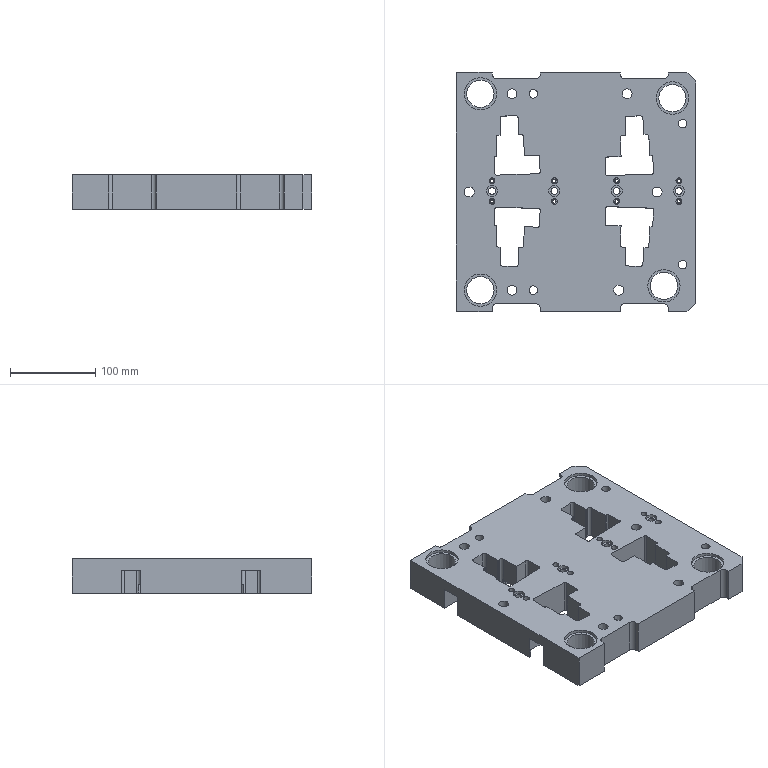Part | NX | features PS-33 2 | 1 solid | 306 faces | box 280 x 280 x 40 mm | volume 2297563 mm3 | plane 160 | cylinder 146 | commonest cylinder face diameters 10 x34 6 x18 8 x18 4 x16 6.4 x12 4.001 x8